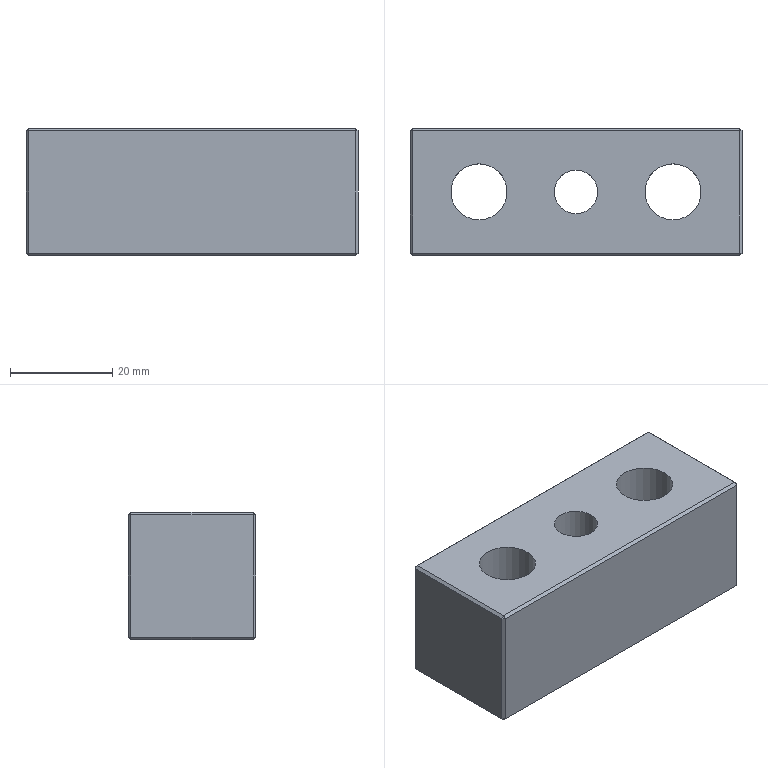Part | NX | features solid 2 | 1 solid | 173 faces | box 65 x 25 x 25 mm | volume 30710 mm3 | plane 126 | spline 41 | cylinder 6 | commonest cylinder face diameters 11 x3 17 x2 8.5 x1